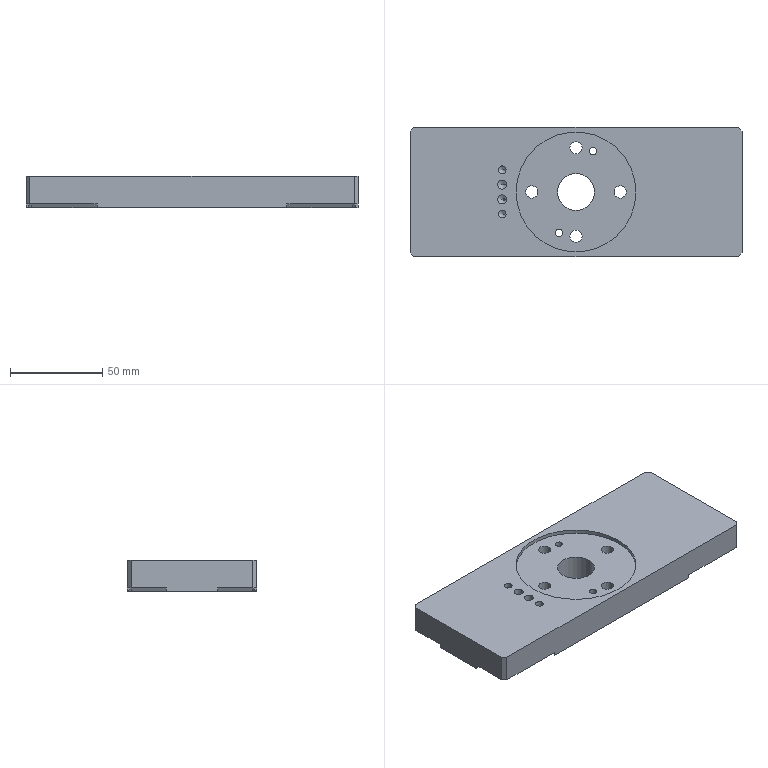Part | STEP file | 11-FG-E01511 | 1 solid | 151 faces | box 180 x 70 x 17 mm | volume 176306 mm3 | plane 71 | cylinder 52 | cone 28 | commonest cylinder face diameters 2 x16 6.6 x8 11 x8 3.3 x4 4 x4 4.2 x4